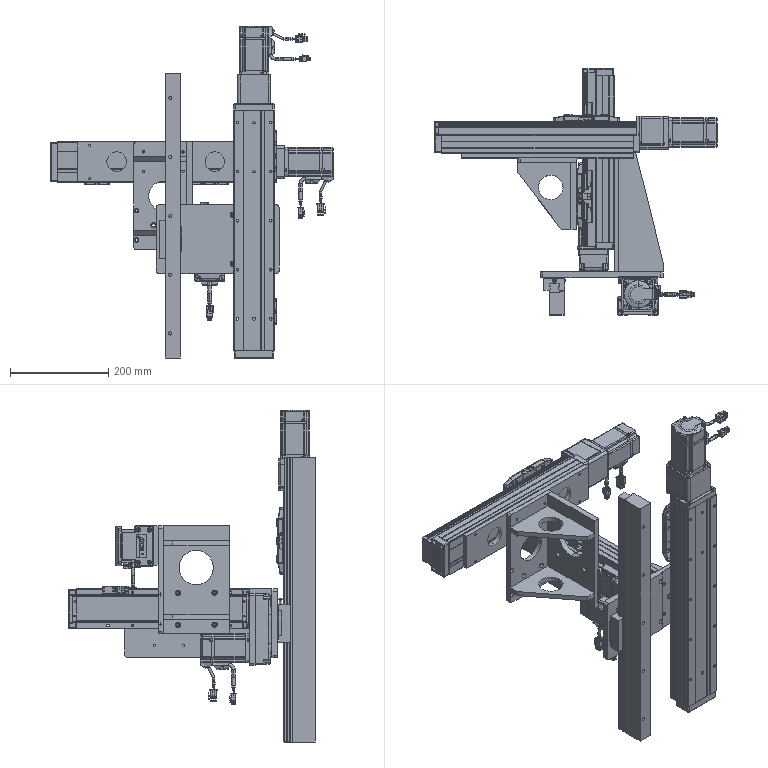Part | SolidWorks | features InContextFeatHolder 20 | 12 solids | 6170 faces | volume 10894817 mm3 | plane 2827 | cylinder 2448 | cone 587 | spline 189 | sphere 78 | torus 41 | commonest cylinder face diameters 1 x327 2 x181 4 x168 6 x141 2.5 x120 8 x114